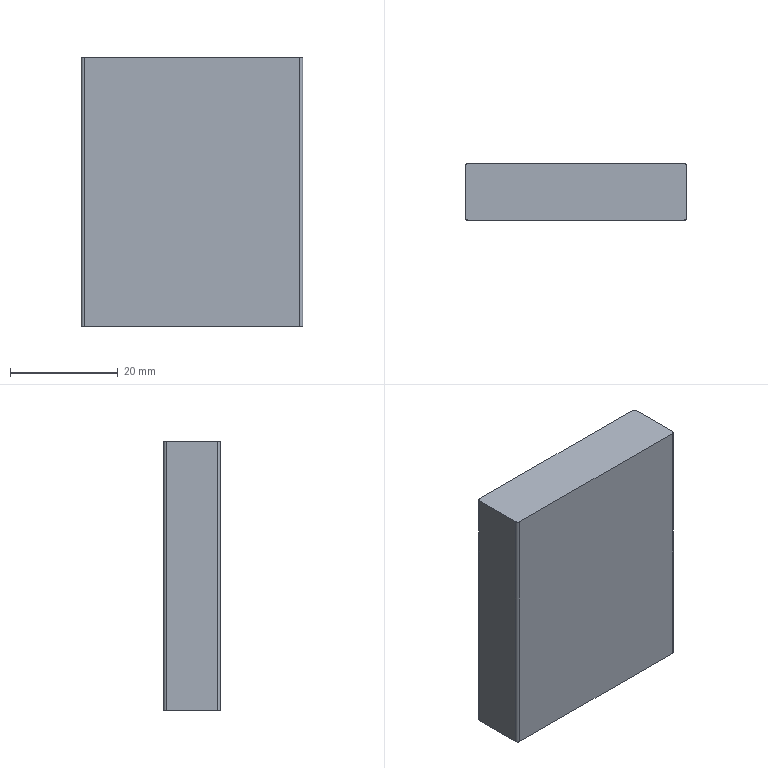Part | NX | features BREP 1 | 1 solid | 10 faces | box 41.1 x 10.507 x 50 mm | volume 21581 mm3 | plane 6 | cylinder 4 | commonest cylinder face diameters 1 x4
STEP:
#1=CARTESIAN_POINT('',(-20.05,5.254,-40.6));
#2=VERTEX_POINT('',#1);
#3=CARTESIAN_POINT('',(-20.55,4.754,-40.6));
#4=VERTEX_POINT('',#3);
#5=CARTESIAN_POINT('',(-20.05,4.754,-40.6));
#6=DIRECTION('',(0.,0.,1.));
#7=DIRECTION('',(1.,0.,0.));
#8=AXIS2_PLACEMENT_3D('',#5,#6,#7);
#9=CIRCLE('',#8,0.5);
#10=EDGE_CURVE('',#2,#4,#9,.T.);
#11=ORIENTED_EDGE('',*,*,#10,.F.);
#12=CARTESIAN_POINT('',(-20.05,5.254,-90.6));
#13=VERTEX_POINT('',#12);
#14=CARTESIAN_POINT('',(-20.05,5.254,-90.6));
#15=DIRECTION('',(0.,0.,1.));
#16=VECTOR('',#15,1000.);
#17=LINE('',#14,#16);
#18=EDGE_CURVE('',#13,#2,#17,.T.);
#19=ORIENTED_EDGE('',*,*,#18,.F.);
#20=CARTESIAN_POINT('',(-20.55,4.754,-90.6));
#21=VERTEX_POINT('',#20);
#22=CARTESIAN_POINT('',(-20.05,4.754,-90.6));
#23=DIRECTION('',(0.,0.,1.));
#24=DIRECTION('',(1.,0.,0.));
#25=AXIS2_PLACEMENT_3D('',#22,#23,#24);
#26=CIRCLE('',#25,0.5);
#27=EDGE_CURVE('',#13,#21,#26,.T.);
#28=ORIENTED_EDGE('',*,*,#27,.T.);
#29=CARTESIAN_POINT('',(-20.55,4.754,-90.6));
#30=DIRECTION('',(0.,0.,1.));
#31=VECTOR('',#30,1000.);
#32=LINE('',#29,#31);
#33=EDGE_CURVE('',#21,#4,#32,.T.);
#34=ORIENTED_EDGE('',*,*,#33,.T.);
#35=EDGE_LOOP('',(#11,#19,#28,#34));
#36=FACE_BOUND('',#35,.T.);
#37=CARTESIAN_POINT('',(-20.05,4.754,-90.6));
#38=DIRECTION('',(0.,0.,1.));
#39=DIRECTION('',(-1.,0.,0.));
#40=AXIS2_PLACEMENT_3D('',#37,#38,#39);
#41=CYLINDRICAL_SURFACE('',#40,0.5);
#42=ADVANCED_FACE('',(#36),#41,.T.);
#43=CARTESIAN_POINT('',(-20.55,-4.754,-40.6));
#44=VERTEX_POINT('',#43);
#45=CARTESIAN_POINT('',(-20.55,-4.754,-40.6));
#46=DIRECTION('',(0.,1.,0.));
#47=VECTOR('',#46,1000.);
#48=LINE('',#45,#47);
#49=EDGE_CURVE('',#44,#4,#48,.T.);
#50=ORIENTED_EDGE('',*,*,#49,.T.);
#51=ORIENTED_EDGE('',*,*,#33,.F.);
#52=CARTESIAN_POINT('',(-20.55,-4.754,-90.6));
#53=VERTEX_POINT('',#52);
#54=CARTESIAN_POINT('',(-20.55,-4.754,-90.6));
#55=DIRECTION('',(0.,1.,0.));
#56=VECTOR('',#55,1000.);
#57=LINE('',#54,#56);
#58=EDGE_CURVE('',#53,#21,#57,.T.);
#59=ORIENTED_EDGE('',*,*,#58,.F.);
#60=CARTESIAN_POINT('',(-20.55,-4.754,-90.6));
#61=DIRECTION('',(0.,0.,1.));
#62=VECTOR('',#61,1000.);
#63=LINE('',#60,#62);
#64=EDGE_CURVE('',#53,#44,#63,.T.);
#65=ORIENTED_EDGE('',*,*,#64,.T.);
#66=EDGE_LOOP('',(#50,#51,#59,#65));
#67=FACE_BOUND('',#66,.T.);
#68=CARTESIAN_POINT('',(-20.55,-4.754,-90.6));
#69=DIRECTION('',(1.,0.,0.));
#70=DIRECTION('',(0.,0.,1.));
#71=AXIS2_PLACEMENT_3D('',#68,#69,#70);
#72=PLANE('',#71);
#73=ADVANCED_FACE('',(#67),#72,.F.);
#74=CARTESIAN_POINT('',(-20.05,-5.254,-40.6));
#75=VERTEX_POINT('',#74);
#76=CARTESIAN_POINT('',(-20.05,-4.754,-40.6));
#77=DIRECTION('',(0.,0.,1.));
#78=DIRECTION('',(1.,0.,0.));
#79=AXIS2_PLACEMENT_3D('',#76,#77,#78);
#80=CIRCLE('',#79,0.5);
#81=EDGE_CURVE('',#44,#75,#80,.T.);
#82=ORIENTED_EDGE('',*,*,#81,.F.);
#83=ORIENTED_EDGE('',*,*,#64,.F.);
#84=CARTESIAN_POINT('',(-20.05,-5.254,-90.6));
#85=VERTEX_POINT('',#84);
#86=CARTESIAN_POINT('',(-20.05,-4.754,-90.6));
#87=DIRECTION('',(0.,0.,1.));
#88=DIRECTION('',(1.,0.,0.));
#89=AXIS2_PLACEMENT_3D('',#86,#87,#88);
#90=CIRCLE('',#89,0.5);
#91=EDGE_CURVE('',#53,#85,#90,.T.);
#92=ORIENTED_EDGE('',*,*,#91,.T.);
#93=CARTESIAN_POINT('',(-20.05,-5.254,-90.6));
#94=DIRECTION('',(0.,0.,1.));
#95=VECTOR('',#94,1000.);
#96=LINE('',#93,#95);
#97=EDGE_CURVE('',#85,#75,#96,.T.);
#98=ORIENTED_EDGE('',*,*,#97,.T.);
#99=EDGE_LOOP('',(#82,#83,#92,#98));
#100=FACE_BOUND('',#99,.T.);
#101=CARTESIAN_POINT('',(-20.05,-4.754,-90.6));
#102=DIRECTION('',(0.,0.,1.));
#103=DIRECTION('',(-1.,0.,0.));
#104=AXIS2_PLACEMENT_3D('',#101,#102,#103);
#105=CYLINDRICAL_SURFACE('',#104,0.5);
#106=ADVANCED_FACE('',(#100),#105,.T.);
#107=CARTESIAN_POINT('',(20.05,-5.254,-40.6));
#108=VERTEX_POINT('',#107);
#109=CARTESIAN_POINT('',(20.05,-5.254,-40.6));
#110=DIRECTION('',(-1.,0.,0.));
#111=VECTOR('',#110,1000.);
#112=LINE('',#109,#111);
#113=EDGE_CURVE('',#108,#75,#112,.T.);
#114=ORIENTED_EDGE('',*,*,#113,.T.);
#115=ORIENTED_EDGE('',*,*,#97,.F.);
#116=CARTESIAN_POINT('',(20.05,-5.254,-90.6));
#117=VERTEX_POINT('',#116);
#118=CARTESIAN_POINT('',(20.05,-5.254,-90.6));
#119=DIRECTION('',(-1.,0.,0.));
#120=VECTOR('',#119,1000.);
#121=LINE('',#118,#120);
#122=EDGE_CURVE('',#117,#85,#121,.T.);
#123=ORIENTED_EDGE('',*,*,#122,.F.);
#124=CARTESIAN_POINT('',(20.05,-5.254,-90.6));
#125=DIRECTION('',(0.,0.,1.));
#126=VECTOR('',#125,1000.);
#127=LINE('',#124,#126);
#128=EDGE_CURVE('',#117,#108,#127,.T.);
#129=ORIENTED_EDGE('',*,*,#128,.T.);
#130=EDGE_LOOP('',(#114,#115,#123,#129));
#131=FACE_BOUND('',#130,.T.);
#132=CARTESIAN_POINT('',(20.05,-5.254,-90.6));
#133=DIRECTION('',(0.,1.,0.));
#134=DIRECTION('',(1.,0.,0.));
#135=AXIS2_PLACEMENT_3D('',#132,#133,#134);
#136=PLANE('',#135);
#137=ADVANCED_FACE('',(#131),#136,.F.);
#138=CARTESIAN_POINT('',(20.55,-4.754,-40.6));
#139=VERTEX_POINT('',#138);
#140=CARTESIAN_POINT('',(20.05,-4.754,-40.6));
#141=DIRECTION('',(0.,0.,1.));
#142=DIRECTION('',(1.,0.,0.));
#143=AXIS2_PLACEMENT_3D('',#140,#141,#142);
#144=CIRCLE('',#143,0.5);
#145=EDGE_CURVE('',#108,#139,#144,.T.);
#146=ORIENTED_EDGE('',*,*,#145,.F.);
#147=ORIENTED_EDGE('',*,*,#128,.F.);
#148=CARTESIAN_POINT('',(20.55,-4.754,-90.6));
#149=VERTEX_POINT('',#148);
#150=CARTESIAN_POINT('',(20.05,-4.754,-90.6));
#151=DIRECTION('',(0.,0.,1.));
#152=DIRECTION('',(1.,0.,0.));
#153=AXIS2_PLACEMENT_3D('',#150,#151,#152);
#154=CIRCLE('',#153,0.5);
#155=EDGE_CURVE('',#117,#149,#154,.T.);
#156=ORIENTED_EDGE('',*,*,#155,.T.);
#157=CARTESIAN_POINT('',(20.55,-4.754,-90.6));
#158=DIRECTION('',(0.,0.,1.));
#159=VECTOR('',#158,1000.);
#160=LINE('',#157,#159);
#161=EDGE_CURVE('',#149,#139,#160,.T.);
#162=ORIENTED_EDGE('',*,*,#161,.T.);
#163=EDGE_LOOP('',(#146,#147,#156,#162));
#164=FACE_BOUND('',#163,.T.);
#165=CARTESIAN_POINT('',(20.05,-4.754,-90.6));
#166=DIRECTION('',(0.,0.,1.));
#167=DIRECTION('',(-1.,0.,0.));
#168=AXIS2_PLACEMENT_3D('',#165,#166,#167);
#169=CYLINDRICAL_SURFACE('',#168,0.5);
#170=ADVANCED_FACE('',(#164),#169,.T.);
#171=CARTESIAN_POINT('',(20.55,4.754,-40.6));
#172=VERTEX_POINT('',#171);
#173=CARTESIAN_POINT('',(20.55,4.754,-40.6));
#174=DIRECTION('',(0.,-1.,0.));
#175=VECTOR('',#174,1000.);
#176=LINE('',#173,#175);
#177=EDGE_CURVE('',#172,#139,#176,.T.);
#178=ORIENTED_EDGE('',*,*,#177,.T.);
#179=ORIENTED_EDGE('',*,*,#161,.F.);
#180=CARTESIAN_POINT('',(20.55,4.754,-90.6));
#181=VERTEX_POINT('',#180);
#182=CARTESIAN_POINT('',(20.55,4.754,-90.6));
#183=DIRECTION('',(0.,-1.,0.));
#184=VECTOR('',#183,1000.);
#185=LINE('',#182,#184);
#186=EDGE_CURVE('',#181,#149,#185,.T.);
#187=ORIENTED_EDGE('',*,*,#186,.F.);
#188=CARTESIAN_POINT('',(20.55,4.754,-90.6));
#189=DIRECTION('',(0.,0.,1.));
#190=VECTOR('',#189,1000.);
#191=LINE('',#188,#190);
#192=EDGE_CURVE('',#181,#172,#191,.T.);
#193=ORIENTED_EDGE('',*,*,#192,.T.);
#194=EDGE_LOOP('',(#178,#179,#187,#193));
#195=FACE_BOUND('',#194,.T.);
#196=CARTESIAN_POINT('',(20.55,4.754,-90.6));
#197=DIRECTION('',(-1.,0.,0.));
#198=DIRECTION('',(0.,1.,0.));
#199=AXIS2_PLACEMENT_3D('',#196,#197,#198);
#200=PLANE('',#199);
#201=ADVANCED_FACE('',(#195),#200,.F.);
#202=CARTESIAN_POINT('',(20.05,5.254,-40.6));
#203=VERTEX_POINT('',#202);
#204=CARTESIAN_POINT('',(20.05,4.754,-40.6));
#205=DIRECTION('',(0.,0.,1.));
#206=DIRECTION('',(1.,0.,0.));
#207=AXIS2_PLACEMENT_3D('',#204,#205,#206);
#208=CIRCLE('',#207,0.5);
#209=EDGE_CURVE('',#172,#203,#208,.T.);
#210=ORIENTED_EDGE('',*,*,#209,.F.);
#211=ORIENTED_EDGE('',*,*,#192,.F.);
#212=CARTESIAN_POINT('',(20.05,5.254,-90.6));
#213=VERTEX_POINT('',#212);
#214=CARTESIAN_POINT('',(20.05,4.754,-90.6));
#215=DIRECTION('',(0.,0.,1.));
#216=DIRECTION('',(1.,0.,0.));
#217=AXIS2_PLACEMENT_3D('',#214,#215,#216);
#218=CIRCLE('',#217,0.5);
#219=EDGE_CURVE('',#181,#213,#218,.T.);
#220=ORIENTED_EDGE('',*,*,#219,.T.);
#221=CARTESIAN_POINT('',(20.05,5.254,-90.6));
#222=DIRECTION('',(0.,0.,1.));
#223=VECTOR('',#222,1000.);
#224=LINE('',#221,#223);
#225=EDGE_CURVE('',#213,#203,#224,.T.);
#226=ORIENTED_EDGE('',*,*,#225,.T.);
#227=EDGE_LOOP('',(#210,#211,#220,#226));
#228=FACE_BOUND('',#227,.T.);
#229=CARTESIAN_POINT('',(20.05,4.754,-90.6));
#230=DIRECTION('',(0.,0.,1.));
#231=DIRECTION('',(-1.,0.,0.));
#232=AXIS2_PLACEMENT_3D('',#229,#230,#231);
#233=CYLINDRICAL_SURFACE('',#232,0.5);
#234=ADVANCED_FACE('',(#228),#233,.T.);
#235=CARTESIAN_POINT('',(-20.05,5.254,-40.6));
#236=DIRECTION('',(1.,0.,0.));
#237=VECTOR('',#236,1000.);
#238=LINE('',#235,#237);
#239=EDGE_CURVE('',#2,#203,#238,.T.);
#240=ORIENTED_EDGE('',*,*,#239,.T.);
#241=ORIENTED_EDGE('',*,*,#225,.F.);
#242=CARTESIAN_POINT('',(-20.05,5.254,-90.6));
#243=DIRECTION('',(1.,0.,0.));
#244=VECTOR('',#243,1000.);
#245=LINE('',#242,#244);
#246=EDGE_CURVE('',#13,#213,#245,.T.);
#247=ORIENTED_EDGE('',*,*,#246,.F.);
#248=ORIENTED_EDGE('',*,*,#18,.T.);
#249=EDGE_LOOP('',(#240,#241,#247,#248));
#250=FACE_BOUND('',#249,.T.);
#251=CARTESIAN_POINT('',(-20.05,5.254,-90.6));
#252=DIRECTION('',(0.,-1.,0.));
#253=DIRECTION('',(0.,0.,1.));
#254=AXIS2_PLACEMENT_3D('',#251,#252,#253);
#255=PLANE('',#254);
#256=ADVANCED_FACE('',(#250),#255,.F.);
#257=ORIENTED_EDGE('',*,*,#27,.F.);
#258=ORIENTED_EDGE('',*,*,#246,.T.);
#259=ORIENTED_EDGE('',*,*,#219,.F.);
#260=ORIENTED_EDGE('',*,*,#186,.T.);
#261=ORIENTED_EDGE('',*,*,#155,.F.);
#262=ORIENTED_EDGE('',*,*,#122,.T.);
#263=ORIENTED_EDGE('',*,*,#91,.F.);
#264=ORIENTED_EDGE('',*,*,#58,.T.);
#265=EDGE_LOOP('',(#257,#258,#259,#260,#261,#262,#263,#264));
#266=FACE_BOUND('',#265,.T.);
#267=CARTESIAN_POINT('',(-20.05,4.754,-90.6));
#268=DIRECTION('',(0.,0.,1.));
#269=DIRECTION('',(-1.,0.,0.));
#270=AXIS2_PLACEMENT_3D('',#267,#268,#269);
#271=PLANE('',#270);
#272=ADVANCED_FACE('',(#266),#271,.F.);
#273=ORIENTED_EDGE('',*,*,#10,.T.);
#274=ORIENTED_EDGE('',*,*,#49,.F.);
#275=ORIENTED_EDGE('',*,*,#81,.T.);
#276=ORIENTED_EDGE('',*,*,#113,.F.);
#277=ORIENTED_EDGE('',*,*,#145,.T.);
#278=ORIENTED_EDGE('',*,*,#177,.F.);
#279=ORIENTED_EDGE('',*,*,#209,.T.);
#280=ORIENTED_EDGE('',*,*,#239,.F.);
#281=EDGE_LOOP('',(#273,#274,#275,#276,#277,#278,#279,#280));
#282=FACE_BOUND('',#281,.T.);
#283=CARTESIAN_POINT('',(-20.05,4.754,-40.6));
#284=DIRECTION('',(0.,0.,1.));
#285=DIRECTION('',(-1.,0.,0.));
#286=AXIS2_PLACEMENT_3D('',#283,#284,#285);
#287=PLANE('',#286);
#288=ADVANCED_FACE('',(#282),#287,.T.);
#289=CLOSED_SHELL('',(#42,#73,#106,#137,#170,#201,#234,#256,#272,#288));
#290=MANIFOLD_SOLID_BREP('',#289);
#291=(LENGTH_UNIT()NAMED_UNIT(*)SI_UNIT(.MILLI.,.METRE.));
#292=UNCERTAINTY_MEASURE_WITH_UNIT(LENGTH_MEASURE(0.00001),#291,'','');
#293=(NAMED_UNIT(*)PLANE_ANGLE_UNIT()SI_UNIT($,.RADIAN.));
#294=(NAMED_UNIT(*)SI_UNIT($,.STERADIAN.)SOLID_ANGLE_UNIT());
#295=(GEOMETRIC_REPRESENTATION_CONTEXT(3)GLOBAL_UNCERTAINTY_ASSIGNED_CONTEXT((#292))GLOBAL_UNIT_ASSIGNED_CONTEXT((#291,#293,#294))REPRESENTATION_CONTEXT('',''));
#296=ADVANCED_BREP_SHAPE_REPRESENTATION('',(#290),#295);